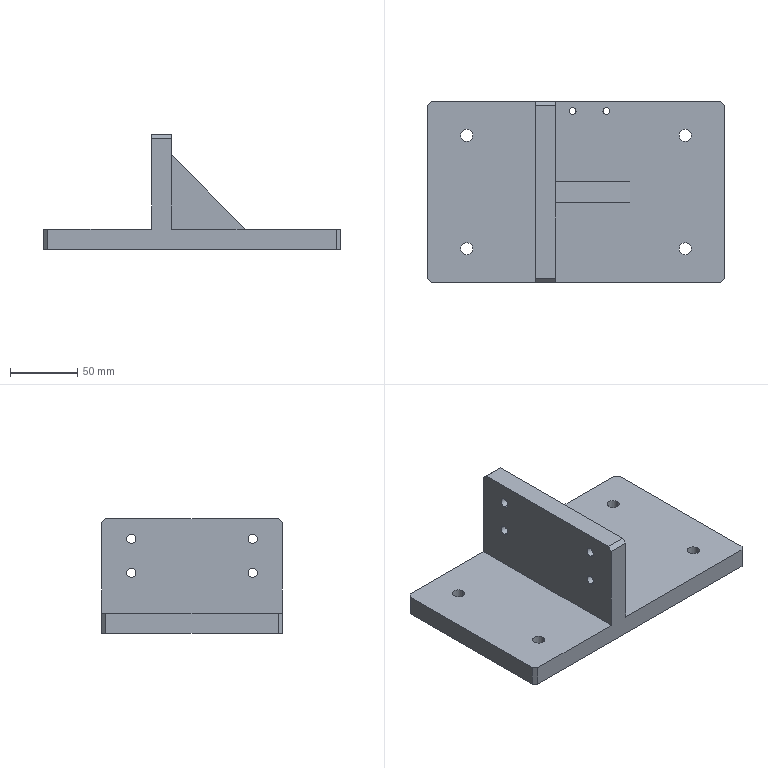Part | STEP file | 2 solids | 41 faces | box 220 x 134 x 85 mm | volume 598597 mm3 | plane 21 | cylinder 20 | commonest cylinder face diameters 6.8 x8 9 x8 5 x4